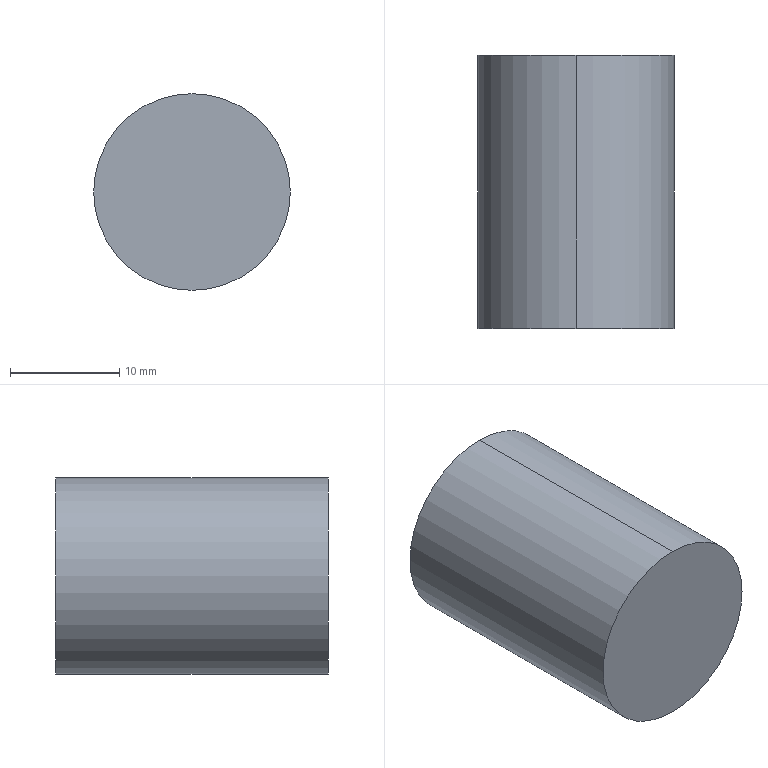Part | SolidWorks | features Extrusion 1 | 1 solid | 4 faces | box 18 x 25 x 18 mm | volume 6362 mm3 | cylinder 2 | plane 2 | commonest cylinder face diameters 18 x2
STEP:
#1=CARTESIAN_POINT('',(0.,12.5,9.));
#2=VERTEX_POINT('',#1);
#3=CARTESIAN_POINT('',(0.,12.5,-9.));
#4=VERTEX_POINT('',#3);
#5=CARTESIAN_POINT('',(0.,12.5,0.));
#6=DIRECTION('',(0.,1.,0.));
#7=DIRECTION('',(0.,0.,1.));
#8=AXIS2_PLACEMENT_3D('',#5,#6,#7);
#9=CIRCLE('',#8,9.);
#10=EDGE_CURVE('',#2,#4,#9,.T.);
#11=ORIENTED_EDGE('',*,*,#10,.F.);
#12=CARTESIAN_POINT('',(0.,-12.5,9.));
#13=VERTEX_POINT('',#12);
#14=CARTESIAN_POINT('',(0.,12.5,9.));
#15=DIRECTION('',(0.,-1.,0.));
#16=VECTOR('',#15,1000.);
#17=LINE('',#14,#16);
#18=EDGE_CURVE('',#2,#13,#17,.T.);
#19=ORIENTED_EDGE('',*,*,#18,.T.);
#20=CARTESIAN_POINT('',(0.,-12.5,-9.));
#21=VERTEX_POINT('',#20);
#22=CARTESIAN_POINT('',(0.,-12.5,0.));
#23=DIRECTION('',(0.,1.,0.));
#24=DIRECTION('',(0.,0.,1.));
#25=AXIS2_PLACEMENT_3D('',#22,#23,#24);
#26=CIRCLE('',#25,9.);
#27=EDGE_CURVE('',#13,#21,#26,.T.);
#28=ORIENTED_EDGE('',*,*,#27,.T.);
#29=CARTESIAN_POINT('',(0.,12.5,-9.));
#30=DIRECTION('',(0.,-1.,0.));
#31=VECTOR('',#30,1000.);
#32=LINE('',#29,#31);
#33=EDGE_CURVE('',#4,#21,#32,.T.);
#34=ORIENTED_EDGE('',*,*,#33,.F.);
#35=EDGE_LOOP('',(#11,#19,#28,#34));
#36=FACE_OUTER_BOUND('',#35,.T.);
#37=CARTESIAN_POINT('',(0.,12.5,0.));
#38=DIRECTION('',(0.,-1.,0.));
#39=DIRECTION('',(0.,0.,-1.));
#40=AXIS2_PLACEMENT_3D('',#37,#38,#39);
#41=CYLINDRICAL_SURFACE('',#40,9.);
#42=ADVANCED_FACE('',(#36),#41,.T.);
#43=ORIENTED_EDGE('',*,*,#18,.F.);
#44=CARTESIAN_POINT('',(0.,12.5,0.));
#45=DIRECTION('',(0.,1.,0.));
#46=DIRECTION('',(0.,0.,1.));
#47=AXIS2_PLACEMENT_3D('',#44,#45,#46);
#48=CIRCLE('',#47,9.);
#49=EDGE_CURVE('',#4,#2,#48,.T.);
#50=ORIENTED_EDGE('',*,*,#49,.F.);
#51=ORIENTED_EDGE('',*,*,#33,.T.);
#52=CARTESIAN_POINT('',(0.,-12.5,0.));
#53=DIRECTION('',(0.,1.,0.));
#54=DIRECTION('',(0.,0.,1.));
#55=AXIS2_PLACEMENT_3D('',#52,#53,#54);
#56=CIRCLE('',#55,9.);
#57=EDGE_CURVE('',#21,#13,#56,.T.);
#58=ORIENTED_EDGE('',*,*,#57,.T.);
#59=EDGE_LOOP('',(#43,#50,#51,#58));
#60=FACE_OUTER_BOUND('',#59,.T.);
#61=CARTESIAN_POINT('',(0.,12.5,0.));
#62=DIRECTION('',(0.,-1.,0.));
#63=DIRECTION('',(0.,0.,-1.));
#64=AXIS2_PLACEMENT_3D('',#61,#62,#63);
#65=CYLINDRICAL_SURFACE('',#64,9.);
#66=ADVANCED_FACE('',(#60),#65,.T.);
#67=ORIENTED_EDGE('',*,*,#49,.T.);
#68=ORIENTED_EDGE('',*,*,#10,.T.);
#69=EDGE_LOOP('',(#67,#68));
#70=FACE_OUTER_BOUND('',#69,.T.);
#71=CARTESIAN_POINT('',(0.,12.5,0.));
#72=DIRECTION('',(0.,1.,0.));
#73=DIRECTION('',(0.,0.,1.));
#74=AXIS2_PLACEMENT_3D('',#71,#72,#73);
#75=PLANE('',#74);
#76=ADVANCED_FACE('',(#70),#75,.T.);
#77=ORIENTED_EDGE('',*,*,#57,.F.);
#78=ORIENTED_EDGE('',*,*,#27,.F.);
#79=EDGE_LOOP('',(#77,#78));
#80=FACE_OUTER_BOUND('',#79,.T.);
#81=CARTESIAN_POINT('',(0.,-12.5,0.));
#82=DIRECTION('',(0.,1.,0.));
#83=DIRECTION('',(0.,0.,1.));
#84=AXIS2_PLACEMENT_3D('',#81,#82,#83);
#85=PLANE('',#84);
#86=ADVANCED_FACE('',(#80),#85,.F.);
#87=CLOSED_SHELL('',(#42,#66,#76,#86));
#88=MANIFOLD_SOLID_BREP('',#87);
#89=CARTESIAN_POINT('',(0.,0.,0.));
#90=DIRECTION('',(0.,0.,1.));
#91=DIRECTION('',(1.,0.,0.));
#92=AXIS2_PLACEMENT_3D('',#89,#90,#91);
#93=(LENGTH_UNIT()NAMED_UNIT(*)SI_UNIT(.MILLI.,.METRE.));
#94=UNCERTAINTY_MEASURE_WITH_UNIT(LENGTH_MEASURE(0.00001),#93,'','');
#95=(NAMED_UNIT(*)PLANE_ANGLE_UNIT()SI_UNIT($,.RADIAN.));
#96=(NAMED_UNIT(*)SI_UNIT($,.STERADIAN.)SOLID_ANGLE_UNIT());
#97=(GEOMETRIC_REPRESENTATION_CONTEXT(3)GLOBAL_UNCERTAINTY_ASSIGNED_CONTEXT((#94))GLOBAL_UNIT_ASSIGNED_CONTEXT((#93,#95,#96))REPRESENTATION_CONTEXT('',''));
#98=ADVANCED_BREP_SHAPE_REPRESENTATION('',(#88,#92),#97);